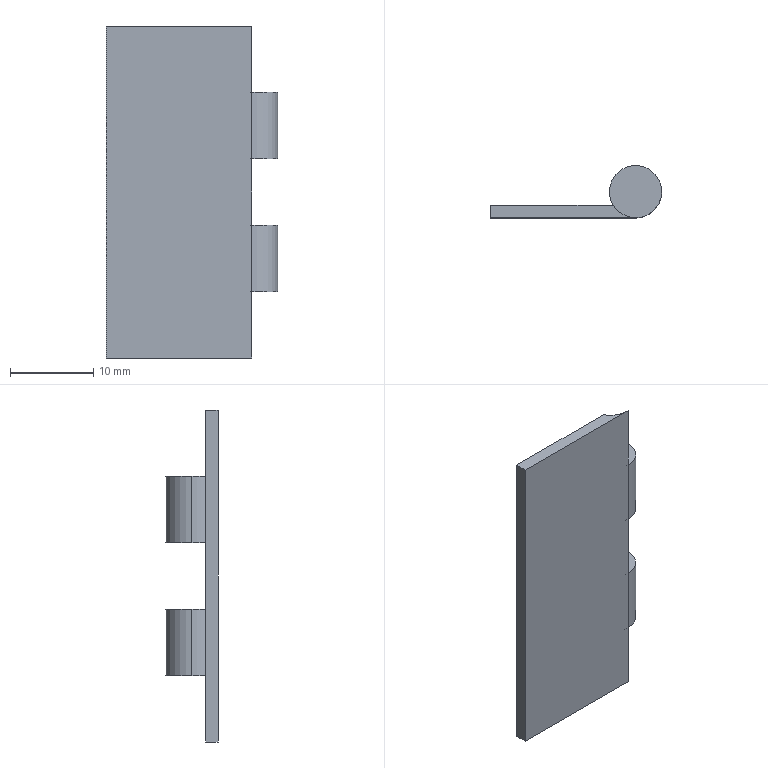Part | SolidWorks | features BaseBody 1 | 1 solid | 18 faces | box 20.65 x 6.3 x 40 mm | volume 1435 mm3 | cylinder 9 | plane 9 | commonest cylinder face diameters 6.3 x9
STEP:
#1=CARTESIAN_POINT('',(3.15,3.15,8.));
#2=VERTEX_POINT('',#1);
#3=CARTESIAN_POINT('',(-3.15,3.15,8.));
#4=VERTEX_POINT('',#3);
#5=CARTESIAN_POINT('',(0.,3.15,8.));
#6=DIRECTION('',(0.,0.,1.));
#7=DIRECTION('',(1.,0.,0.));
#8=AXIS2_PLACEMENT_3D('',#5,#6,#7);
#9=CIRCLE('',#8,3.15);
#10=EDGE_CURVE('',#2,#4,#9,.T.);
#11=ORIENTED_EDGE('',*,*,#10,.T.);
#12=CARTESIAN_POINT('',(-3.15,3.15,16.));
#13=VERTEX_POINT('',#12);
#14=CARTESIAN_POINT('',(-3.15,3.15,40.));
#15=DIRECTION('',(0.,0.,1.));
#16=VECTOR('',#15,1000.);
#17=LINE('',#14,#16);
#18=EDGE_CURVE('',#4,#13,#17,.T.);
#19=ORIENTED_EDGE('',*,*,#18,.T.);
#20=CARTESIAN_POINT('',(3.15,3.15,16.));
#21=VERTEX_POINT('',#20);
#22=CARTESIAN_POINT('',(0.,3.15,16.));
#23=DIRECTION('',(0.,0.,-1.));
#24=DIRECTION('',(1.,0.,0.));
#25=AXIS2_PLACEMENT_3D('',#22,#23,#24);
#26=CIRCLE('',#25,3.15);
#27=EDGE_CURVE('',#13,#21,#26,.T.);
#28=ORIENTED_EDGE('',*,*,#27,.T.);
#29=CARTESIAN_POINT('',(3.15,3.15,40.));
#30=DIRECTION('',(0.,0.,1.));
#31=VECTOR('',#30,1000.);
#32=LINE('',#29,#31);
#33=EDGE_CURVE('',#2,#21,#32,.T.);
#34=ORIENTED_EDGE('',*,*,#33,.F.);
#35=EDGE_LOOP('',(#11,#19,#28,#34));
#36=FACE_OUTER_BOUND('',#35,.T.);
#37=CARTESIAN_POINT('',(0.,3.15,40.));
#38=DIRECTION('',(0.,0.,1.));
#39=DIRECTION('',(1.,0.,0.));
#40=AXIS2_PLACEMENT_3D('',#37,#38,#39);
#41=CYLINDRICAL_SURFACE('',#40,3.15);
#42=ADVANCED_FACE('',(#36),#41,.T.);
#43=CARTESIAN_POINT('',(0.,0.,8.));
#44=VERTEX_POINT('',#43);
#45=CARTESIAN_POINT('',(0.,3.15,8.));
#46=DIRECTION('',(0.,0.,1.));
#47=DIRECTION('',(1.,0.,0.));
#48=AXIS2_PLACEMENT_3D('',#45,#46,#47);
#49=CIRCLE('',#48,3.15);
#50=EDGE_CURVE('',#44,#2,#49,.T.);
#51=ORIENTED_EDGE('',*,*,#50,.T.);
#52=ORIENTED_EDGE('',*,*,#33,.T.);
#53=CARTESIAN_POINT('',(0.,0.,16.));
#54=VERTEX_POINT('',#53);
#55=CARTESIAN_POINT('',(0.,3.15,16.));
#56=DIRECTION('',(0.,0.,-1.));
#57=DIRECTION('',(1.,0.,0.));
#58=AXIS2_PLACEMENT_3D('',#55,#56,#57);
#59=CIRCLE('',#58,3.15);
#60=EDGE_CURVE('',#21,#54,#59,.T.);
#61=ORIENTED_EDGE('',*,*,#60,.T.);
#62=CARTESIAN_POINT('',(0.,0.,40.));
#63=DIRECTION('',(0.,0.,-1.));
#64=VECTOR('',#63,1000.);
#65=LINE('',#62,#64);
#66=EDGE_CURVE('',#54,#44,#65,.T.);
#67=ORIENTED_EDGE('',*,*,#66,.T.);
#68=EDGE_LOOP('',(#51,#52,#61,#67));
#69=FACE_OUTER_BOUND('',#68,.T.);
#70=CARTESIAN_POINT('',(0.,3.15,40.));
#71=DIRECTION('',(0.,0.,1.));
#72=DIRECTION('',(1.,0.,0.));
#73=AXIS2_PLACEMENT_3D('',#70,#71,#72);
#74=CYLINDRICAL_SURFACE('',#73,3.15);
#75=ADVANCED_FACE('',(#69),#74,.T.);
#76=CARTESIAN_POINT('',(3.15,3.15,24.));
#77=VERTEX_POINT('',#76);
#78=CARTESIAN_POINT('',(-3.15,3.15,24.));
#79=VERTEX_POINT('',#78);
#80=CARTESIAN_POINT('',(0.,3.15,24.));
#81=DIRECTION('',(0.,0.,1.));
#82=DIRECTION('',(1.,0.,0.));
#83=AXIS2_PLACEMENT_3D('',#80,#81,#82);
#84=CIRCLE('',#83,3.15);
#85=EDGE_CURVE('',#77,#79,#84,.T.);
#86=ORIENTED_EDGE('',*,*,#85,.T.);
#87=CARTESIAN_POINT('',(-3.15,3.15,32.));
#88=VERTEX_POINT('',#87);
#89=CARTESIAN_POINT('',(-3.15,3.15,40.));
#90=DIRECTION('',(0.,0.,1.));
#91=VECTOR('',#90,1000.);
#92=LINE('',#89,#91);
#93=EDGE_CURVE('',#79,#88,#92,.T.);
#94=ORIENTED_EDGE('',*,*,#93,.T.);
#95=CARTESIAN_POINT('',(3.15,3.15,32.));
#96=VERTEX_POINT('',#95);
#97=CARTESIAN_POINT('',(0.,3.15,32.));
#98=DIRECTION('',(0.,0.,-1.));
#99=DIRECTION('',(1.,0.,0.));
#100=AXIS2_PLACEMENT_3D('',#97,#98,#99);
#101=CIRCLE('',#100,3.15);
#102=EDGE_CURVE('',#88,#96,#101,.T.);
#103=ORIENTED_EDGE('',*,*,#102,.T.);
#104=CARTESIAN_POINT('',(3.15,3.15,40.));
#105=DIRECTION('',(0.,0.,1.));
#106=VECTOR('',#105,1000.);
#107=LINE('',#104,#106);
#108=EDGE_CURVE('',#77,#96,#107,.T.);
#109=ORIENTED_EDGE('',*,*,#108,.F.);
#110=EDGE_LOOP('',(#86,#94,#103,#109));
#111=FACE_OUTER_BOUND('',#110,.T.);
#112=CARTESIAN_POINT('',(0.,3.15,40.));
#113=DIRECTION('',(0.,0.,1.));
#114=DIRECTION('',(1.,0.,0.));
#115=AXIS2_PLACEMENT_3D('',#112,#113,#114);
#116=CYLINDRICAL_SURFACE('',#115,3.15);
#117=ADVANCED_FACE('',(#111),#116,.T.);
#118=CARTESIAN_POINT('',(0.,0.,24.));
#119=VERTEX_POINT('',#118);
#120=CARTESIAN_POINT('',(0.,3.15,24.));
#121=DIRECTION('',(0.,0.,1.));
#122=DIRECTION('',(1.,0.,0.));
#123=AXIS2_PLACEMENT_3D('',#120,#121,#122);
#124=CIRCLE('',#123,3.15);
#125=EDGE_CURVE('',#119,#77,#124,.T.);
#126=ORIENTED_EDGE('',*,*,#125,.T.);
#127=ORIENTED_EDGE('',*,*,#108,.T.);
#128=CARTESIAN_POINT('',(0.,0.,32.));
#129=VERTEX_POINT('',#128);
#130=CARTESIAN_POINT('',(0.,3.15,32.));
#131=DIRECTION('',(0.,0.,-1.));
#132=DIRECTION('',(1.,0.,0.));
#133=AXIS2_PLACEMENT_3D('',#130,#131,#132);
#134=CIRCLE('',#133,3.15);
#135=EDGE_CURVE('',#96,#129,#134,.T.);
#136=ORIENTED_EDGE('',*,*,#135,.T.);
#137=CARTESIAN_POINT('',(0.,0.,40.));
#138=DIRECTION('',(0.,0.,-1.));
#139=VECTOR('',#138,1000.);
#140=LINE('',#137,#139);
#141=EDGE_CURVE('',#129,#119,#140,.T.);
#142=ORIENTED_EDGE('',*,*,#141,.T.);
#143=EDGE_LOOP('',(#126,#127,#136,#142));
#144=FACE_OUTER_BOUND('',#143,.T.);
#145=CARTESIAN_POINT('',(0.,3.15,40.));
#146=DIRECTION('',(0.,0.,1.));
#147=DIRECTION('',(1.,0.,0.));
#148=AXIS2_PLACEMENT_3D('',#145,#146,#147);
#149=CYLINDRICAL_SURFACE('',#148,3.15);
#150=ADVANCED_FACE('',(#144),#149,.T.);
#151=CARTESIAN_POINT('',(0.,0.,0.));
#152=VERTEX_POINT('',#151);
#153=CARTESIAN_POINT('',(0.,0.,40.));
#154=DIRECTION('',(0.,0.,-1.));
#155=VECTOR('',#154,1000.);
#156=LINE('',#153,#155);
#157=EDGE_CURVE('',#44,#152,#156,.T.);
#158=ORIENTED_EDGE('',*,*,#157,.F.);
#159=ORIENTED_EDGE('',*,*,#66,.F.);
#160=CARTESIAN_POINT('',(0.,0.,40.));
#161=DIRECTION('',(0.,0.,-1.));
#162=VECTOR('',#161,1000.);
#163=LINE('',#160,#162);
#164=EDGE_CURVE('',#119,#54,#163,.T.);
#165=ORIENTED_EDGE('',*,*,#164,.F.);
#166=ORIENTED_EDGE('',*,*,#141,.F.);
#167=CARTESIAN_POINT('',(0.,0.,40.));
#168=VERTEX_POINT('',#167);
#169=CARTESIAN_POINT('',(0.,0.,40.));
#170=DIRECTION('',(0.,0.,-1.));
#171=VECTOR('',#170,1000.);
#172=LINE('',#169,#171);
#173=EDGE_CURVE('',#168,#129,#172,.T.);
#174=ORIENTED_EDGE('',*,*,#173,.F.);
#175=CARTESIAN_POINT('',(-17.5,0.,40.));
#176=VERTEX_POINT('',#175);
#177=CARTESIAN_POINT('',(-17.5,0.,40.));
#178=DIRECTION('',(1.,0.,0.));
#179=VECTOR('',#178,1000.);
#180=LINE('',#177,#179);
#181=EDGE_CURVE('',#176,#168,#180,.T.);
#182=ORIENTED_EDGE('',*,*,#181,.F.);
#183=CARTESIAN_POINT('',(-17.5,0.,0.));
#184=VERTEX_POINT('',#183);
#185=CARTESIAN_POINT('',(-17.5,0.,40.));
#186=DIRECTION('',(0.,0.,1.));
#187=VECTOR('',#186,1000.);
#188=LINE('',#185,#187);
#189=EDGE_CURVE('',#184,#176,#188,.T.);
#190=ORIENTED_EDGE('',*,*,#189,.F.);
#191=CARTESIAN_POINT('',(-17.5,0.,0.));
#192=DIRECTION('',(-1.,0.,0.));
#193=VECTOR('',#192,1000.);
#194=LINE('',#191,#193);
#195=EDGE_CURVE('',#152,#184,#194,.T.);
#196=ORIENTED_EDGE('',*,*,#195,.F.);
#197=EDGE_LOOP('',(#158,#159,#165,#166,#174,#182,#190,#196));
#198=FACE_OUTER_BOUND('',#197,.T.);
#199=CARTESIAN_POINT('',(-17.5,0.,40.));
#200=DIRECTION('',(0.,1.,0.));
#201=DIRECTION('',(0.,0.,1.));
#202=AXIS2_PLACEMENT_3D('',#199,#200,#201);
#203=PLANE('',#202);
#204=ADVANCED_FACE('',(#198),#203,.F.);
#205=ORIENTED_EDGE('',*,*,#195,.T.);
#206=CARTESIAN_POINT('',(-17.5,1.5,0.));
#207=VERTEX_POINT('',#206);
#208=CARTESIAN_POINT('',(-17.5,3.15,0.));
#209=DIRECTION('',(0.,-1.,0.));
#210=VECTOR('',#209,1000.);
#211=LINE('',#208,#210);
#212=EDGE_CURVE('',#207,#184,#211,.T.);
#213=ORIENTED_EDGE('',*,*,#212,.F.);
#214=CARTESIAN_POINT('',(-2.683,1.5,0.));
#215=VERTEX_POINT('',#214);
#216=CARTESIAN_POINT('',(0.,1.5,0.));
#217=DIRECTION('',(-1.,0.,0.));
#218=VECTOR('',#217,1000.);
#219=LINE('',#216,#218);
#220=EDGE_CURVE('',#215,#207,#219,.T.);
#221=ORIENTED_EDGE('',*,*,#220,.F.);
#222=CARTESIAN_POINT('',(0.,3.15,0.));
#223=DIRECTION('',(0.,0.,-1.));
#224=DIRECTION('',(1.,0.,0.));
#225=AXIS2_PLACEMENT_3D('',#222,#223,#224);
#226=CIRCLE('',#225,3.15);
#227=EDGE_CURVE('',#152,#215,#226,.T.);
#228=ORIENTED_EDGE('',*,*,#227,.F.);
#229=EDGE_LOOP('',(#205,#213,#221,#228));
#230=FACE_OUTER_BOUND('',#229,.T.);
#231=CARTESIAN_POINT('',(0.,3.15,0.));
#232=DIRECTION('',(0.,0.,1.));
#233=DIRECTION('',(1.,0.,0.));
#234=AXIS2_PLACEMENT_3D('',#231,#232,#233);
#235=PLANE('',#234);
#236=ADVANCED_FACE('',(#230),#235,.F.);
#237=CARTESIAN_POINT('',(-2.683,1.5,8.));
#238=VERTEX_POINT('',#237);
#239=CARTESIAN_POINT('',(0.,3.15,8.));
#240=DIRECTION('',(0.,0.,-1.));
#241=DIRECTION('',(1.,0.,0.));
#242=AXIS2_PLACEMENT_3D('',#239,#240,#241);
#243=CIRCLE('',#242,3.15);
#244=EDGE_CURVE('',#44,#238,#243,.T.);
#245=ORIENTED_EDGE('',*,*,#244,.F.);
#246=ORIENTED_EDGE('',*,*,#157,.T.);
#247=ORIENTED_EDGE('',*,*,#227,.T.);
#248=CARTESIAN_POINT('',(-2.683,1.5,8.));
#249=DIRECTION('',(0.,0.,-1.));
#250=VECTOR('',#249,1000.);
#251=LINE('',#248,#250);
#252=EDGE_CURVE('',#238,#215,#251,.T.);
#253=ORIENTED_EDGE('',*,*,#252,.F.);
#254=EDGE_LOOP('',(#245,#246,#247,#253));
#255=FACE_OUTER_BOUND('',#254,.T.);
#256=CARTESIAN_POINT('',(0.,3.15,8.));
#257=DIRECTION('',(0.,0.,1.));
#258=DIRECTION('',(1.,0.,0.));
#259=AXIS2_PLACEMENT_3D('',#256,#257,#258);
#260=CYLINDRICAL_SURFACE('',#259,3.15);
#261=ADVANCED_FACE('',(#255),#260,.F.);
#262=ORIENTED_EDGE('',*,*,#18,.F.);
#263=CARTESIAN_POINT('',(0.,3.15,8.));
#264=DIRECTION('',(0.,0.,1.));
#265=DIRECTION('',(1.,0.,0.));
#266=AXIS2_PLACEMENT_3D('',#263,#264,#265);
#267=CIRCLE('',#266,3.15);
#268=EDGE_CURVE('',#4,#238,#267,.T.);
#269=ORIENTED_EDGE('',*,*,#268,.T.);
#270=CARTESIAN_POINT('',(-2.683,1.5,16.));
#271=VERTEX_POINT('',#270);
#272=CARTESIAN_POINT('',(-2.683,1.5,40.));
#273=DIRECTION('',(0.,0.,1.));
#274=VECTOR('',#273,1000.);
#275=LINE('',#272,#274);
#276=EDGE_CURVE('',#238,#271,#275,.T.);
#277=ORIENTED_EDGE('',*,*,#276,.T.);
#278=CARTESIAN_POINT('',(0.,3.15,16.));
#279=DIRECTION('',(0.,0.,-1.));
#280=DIRECTION('',(1.,0.,0.));
#281=AXIS2_PLACEMENT_3D('',#278,#279,#280);
#282=CIRCLE('',#281,3.15);
#283=EDGE_CURVE('',#271,#13,#282,.T.);
#284=ORIENTED_EDGE('',*,*,#283,.T.);
#285=EDGE_LOOP('',(#262,#269,#277,#284));
#286=FACE_OUTER_BOUND('',#285,.T.);
#287=CARTESIAN_POINT('',(0.,3.15,40.));
#288=DIRECTION('',(0.,0.,1.));
#289=DIRECTION('',(1.,0.,0.));
#290=AXIS2_PLACEMENT_3D('',#287,#288,#289);
#291=CYLINDRICAL_SURFACE('',#290,3.15);
#292=ADVANCED_FACE('',(#286),#291,.T.);
#293=CARTESIAN_POINT('',(-2.683,1.5,24.));
#294=VERTEX_POINT('',#293);
#295=CARTESIAN_POINT('',(0.,3.15,24.));
#296=DIRECTION('',(0.,0.,-1.));
#297=DIRECTION('',(1.,0.,0.));
#298=AXIS2_PLACEMENT_3D('',#295,#296,#297);
#299=CIRCLE('',#298,3.15);
#300=EDGE_CURVE('',#119,#294,#299,.T.);
#301=ORIENTED_EDGE('',*,*,#300,.F.);
#302=ORIENTED_EDGE('',*,*,#164,.T.);
#303=CARTESIAN_POINT('',(0.,3.15,16.));
#304=DIRECTION('',(0.,0.,1.));
#305=DIRECTION('',(1.,0.,0.));
#306=AXIS2_PLACEMENT_3D('',#303,#304,#305);
#307=CIRCLE('',#306,3.15);
#308=EDGE_CURVE('',#271,#54,#307,.T.);
#309=ORIENTED_EDGE('',*,*,#308,.F.);
#310=CARTESIAN_POINT('',(-2.683,1.5,24.));
#311=DIRECTION('',(0.,0.,-1.));
#312=VECTOR('',#311,1000.);
#313=LINE('',#310,#312);
#314=EDGE_CURVE('',#294,#271,#313,.T.);
#315=ORIENTED_EDGE('',*,*,#314,.F.);
#316=EDGE_LOOP('',(#301,#302,#309,#315));
#317=FACE_OUTER_BOUND('',#316,.T.);
#318=CARTESIAN_POINT('',(0.,3.15,24.));
#319=DIRECTION('',(0.,0.,1.));
#320=DIRECTION('',(1.,0.,0.));
#321=AXIS2_PLACEMENT_3D('',#318,#319,#320);
#322=CYLINDRICAL_SURFACE('',#321,3.15);
#323=ADVANCED_FACE('',(#317),#322,.F.);
#324=ORIENTED_EDGE('',*,*,#93,.F.);
#325=CARTESIAN_POINT('',(0.,3.15,24.));
#326=DIRECTION('',(0.,0.,1.));
#327=DIRECTION('',(1.,0.,0.));
#328=AXIS2_PLACEMENT_3D('',#325,#326,#327);
#329=CIRCLE('',#328,3.15);
#330=EDGE_CURVE('',#79,#294,#329,.T.);
#331=ORIENTED_EDGE('',*,*,#330,.T.);
#332=CARTESIAN_POINT('',(-2.683,1.5,32.));
#333=VERTEX_POINT('',#332);
#334=CARTESIAN_POINT('',(-2.683,1.5,40.));
#335=DIRECTION('',(0.,0.,1.));
#336=VECTOR('',#335,1000.);
#337=LINE('',#334,#336);
#338=EDGE_CURVE('',#294,#333,#337,.T.);
#339=ORIENTED_EDGE('',*,*,#338,.T.);
#340=CARTESIAN_POINT('',(0.,3.15,32.));
#341=DIRECTION('',(0.,0.,-1.));
#342=DIRECTION('',(1.,0.,0.));
#343=AXIS2_PLACEMENT_3D('',#340,#341,#342);
#344=CIRCLE('',#343,3.15);
#345=EDGE_CURVE('',#333,#88,#344,.T.);
#346=ORIENTED_EDGE('',*,*,#345,.T.);
#347=EDGE_LOOP('',(#324,#331,#339,#346));
#348=FACE_OUTER_BOUND('',#347,.T.);
#349=CARTESIAN_POINT('',(0.,3.15,40.));
#350=DIRECTION('',(0.,0.,1.));
#351=DIRECTION('',(1.,0.,0.));
#352=AXIS2_PLACEMENT_3D('',#349,#350,#351);
#353=CYLINDRICAL_SURFACE('',#352,3.15);
#354=ADVANCED_FACE('',(#348),#353,.T.);
#355=CARTESIAN_POINT('',(-2.683,1.5,40.));
#356=VERTEX_POINT('',#355);
#357=CARTESIAN_POINT('',(0.,3.15,40.));
#358=DIRECTION('',(0.,0.,-1.));
#359=DIRECTION('',(1.,0.,0.));
#360=AXIS2_PLACEMENT_3D('',#357,#358,#359);
#361=CIRCLE('',#360,3.15);
#362=EDGE_CURVE('',#168,#356,#361,.T.);
#363=ORIENTED_EDGE('',*,*,#362,.F.);
#364=ORIENTED_EDGE('',*,*,#173,.T.);
#365=CARTESIAN_POINT('',(0.,3.15,32.));
#366=DIRECTION('',(0.,0.,1.));
#367=DIRECTION('',(1.,0.,0.));
#368=AXIS2_PLACEMENT_3D('',#365,#366,#367);
#369=CIRCLE('',#368,3.15);
#370=EDGE_CURVE('',#333,#129,#369,.T.);
#371=ORIENTED_EDGE('',*,*,#370,.F.);
#372=CARTESIAN_POINT('',(-2.683,1.5,40.));
#373=DIRECTION('',(0.,0.,-1.));
#374=VECTOR('',#373,1000.);
#375=LINE('',#372,#374);
#376=EDGE_CURVE('',#356,#333,#375,.T.);
#377=ORIENTED_EDGE('',*,*,#376,.F.);
#378=EDGE_LOOP('',(#363,#364,#371,#377));
#379=FACE_OUTER_BOUND('',#378,.T.);
#380=CARTESIAN_POINT('',(0.,3.15,40.));
#381=DIRECTION('',(0.,0.,1.));
#382=DIRECTION('',(1.,0.,0.));
#383=AXIS2_PLACEMENT_3D('',#380,#381,#382);
#384=CYLINDRICAL_SURFACE('',#383,3.15);
#385=ADVANCED_FACE('',(#379),#384,.F.);
#386=CARTESIAN_POINT('',(-17.5,1.5,40.));
#387=VERTEX_POINT('',#386);
#388=CARTESIAN_POINT('',(0.,1.5,40.));
#389=DIRECTION('',(-1.,0.,0.));
#390=VECTOR('',#389,1000.);
#391=LINE('',#388,#390);
#392=EDGE_CURVE('',#356,#387,#391,.T.);
#393=ORIENTED_EDGE('',*,*,#392,.T.);
#394=CARTESIAN_POINT('',(-17.5,3.15,40.));
#395=DIRECTION('',(0.,-1.,0.));
#396=VECTOR('',#395,1000.);
#397=LINE('',#394,#396);
#398=EDGE_CURVE('',#387,#176,#397,.T.);
#399=ORIENTED_EDGE('',*,*,#398,.T.);
#400=ORIENTED_EDGE('',*,*,#181,.T.);
#401=ORIENTED_EDGE('',*,*,#362,.T.);
#402=EDGE_LOOP('',(#393,#399,#400,#401));
#403=FACE_OUTER_BOUND('',#402,.T.);
#404=CARTESIAN_POINT('',(0.,3.15,40.));
#405=DIRECTION('',(0.,0.,1.));
#406=DIRECTION('',(1.,0.,0.));
#407=AXIS2_PLACEMENT_3D('',#404,#405,#406);
#408=PLANE('',#407);
#409=ADVANCED_FACE('',(#403),#408,.T.);
#410=ORIENTED_EDGE('',*,*,#189,.T.);
#411=ORIENTED_EDGE('',*,*,#398,.F.);
#412=CARTESIAN_POINT('',(-17.5,1.5,40.));
#413=DIRECTION('',(0.,0.,1.));
#414=VECTOR('',#413,1000.);
#415=LINE('',#412,#414);
#416=EDGE_CURVE('',#207,#387,#415,.T.);
#417=ORIENTED_EDGE('',*,*,#416,.F.);
#418=ORIENTED_EDGE('',*,*,#212,.T.);
#419=EDGE_LOOP('',(#410,#411,#417,#418));
#420=FACE_OUTER_BOUND('',#419,.T.);
#421=CARTESIAN_POINT('',(-17.5,1.5,40.));
#422=DIRECTION('',(1.,0.,0.));
#423=DIRECTION('',(0.,0.,-1.));
#424=AXIS2_PLACEMENT_3D('',#421,#422,#423);
#425=PLANE('',#424);
#426=ADVANCED_FACE('',(#420),#425,.F.);
#427=ORIENTED_EDGE('',*,*,#416,.T.);
#428=ORIENTED_EDGE('',*,*,#392,.F.);
#429=ORIENTED_EDGE('',*,*,#376,.T.);
#430=ORIENTED_EDGE('',*,*,#338,.F.);
#431=ORIENTED_EDGE('',*,*,#314,.T.);
#432=ORIENTED_EDGE('',*,*,#276,.F.);
#433=ORIENTED_EDGE('',*,*,#252,.T.);
#434=ORIENTED_EDGE('',*,*,#220,.T.);
#435=EDGE_LOOP('',(#427,#428,#429,#430,#431,#432,#433,#434));
#436=FACE_OUTER_BOUND('',#435,.T.);
#437=CARTESIAN_POINT('',(-2.683,1.5,40.));
#438=DIRECTION('',(0.,-1.,0.));
#439=DIRECTION('',(0.,0.,-1.));
#440=AXIS2_PLACEMENT_3D('',#437,#438,#439);
#441=PLANE('',#440);
#442=ADVANCED_FACE('',(#436),#441,.F.);
#443=ORIENTED_EDGE('',*,*,#50,.F.);
#444=ORIENTED_EDGE('',*,*,#244,.T.);
#445=ORIENTED_EDGE('',*,*,#268,.F.);
#446=ORIENTED_EDGE('',*,*,#10,.F.);
#447=EDGE_LOOP('',(#443,#444,#445,#446));
#448=FACE_OUTER_BOUND('',#447,.T.);
#449=CARTESIAN_POINT('',(0.,3.15,8.));
#450=DIRECTION('',(0.,0.,1.));
#451=DIRECTION('',(1.,0.,0.));
#452=AXIS2_PLACEMENT_3D('',#449,#450,#451);
#453=PLANE('',#452);
#454=ADVANCED_FACE('',(#448),#453,.F.);
#455=ORIENTED_EDGE('',*,*,#308,.T.);
#456=ORIENTED_EDGE('',*,*,#60,.F.);
#457=ORIENTED_EDGE('',*,*,#27,.F.);
#458=ORIENTED_EDGE('',*,*,#283,.F.);
#459=EDGE_LOOP('',(#455,#456,#457,#458));
#460=FACE_OUTER_BOUND('',#459,.T.);
#461=CARTESIAN_POINT('',(0.,3.15,16.));
#462=DIRECTION('',(0.,0.,1.));
#463=DIRECTION('',(1.,0.,0.));
#464=AXIS2_PLACEMENT_3D('',#461,#462,#463);
#465=PLANE('',#464);
#466=ADVANCED_FACE('',(#460),#465,.T.);
#467=ORIENTED_EDGE('',*,*,#125,.F.);
#468=ORIENTED_EDGE('',*,*,#300,.T.);
#469=ORIENTED_EDGE('',*,*,#330,.F.);
#470=ORIENTED_EDGE('',*,*,#85,.F.);
#471=EDGE_LOOP('',(#467,#468,#469,#470));
#472=FACE_OUTER_BOUND('',#471,.T.);
#473=CARTESIAN_POINT('',(0.,3.15,24.));
#474=DIRECTION('',(0.,0.,1.));
#475=DIRECTION('',(1.,0.,0.));
#476=AXIS2_PLACEMENT_3D('',#473,#474,#475);
#477=PLANE('',#476);
#478=ADVANCED_FACE('',(#472),#477,.F.);
#479=ORIENTED_EDGE('',*,*,#370,.T.);
#480=ORIENTED_EDGE('',*,*,#135,.F.);
#481=ORIENTED_EDGE('',*,*,#102,.F.);
#482=ORIENTED_EDGE('',*,*,#345,.F.);
#483=EDGE_LOOP('',(#479,#480,#481,#482));
#484=FACE_OUTER_BOUND('',#483,.T.);
#485=CARTESIAN_POINT('',(0.,3.15,32.));
#486=DIRECTION('',(0.,0.,1.));
#487=DIRECTION('',(1.,0.,0.));
#488=AXIS2_PLACEMENT_3D('',#485,#486,#487);
#489=PLANE('',#488);
#490=ADVANCED_FACE('',(#484),#489,.T.);
#491=CLOSED_SHELL('',(#42,#75,#117,#150,#204,#236,#261,#292,#323,#354,#385,#409,#426,#442,#454,#466,#478,#490));
#492=MANIFOLD_SOLID_BREP('',#491);
#493=CARTESIAN_POINT('',(0.,0.,0.));
#494=DIRECTION('',(0.,0.,1.));
#495=DIRECTION('',(1.,0.,0.));
#496=AXIS2_PLACEMENT_3D('',#493,#494,#495);
#497=(LENGTH_UNIT()NAMED_UNIT(*)SI_UNIT(.MILLI.,.METRE.));
#498=UNCERTAINTY_MEASURE_WITH_UNIT(LENGTH_MEASURE(0.00001),#497,'','');
#499=(NAMED_UNIT(*)PLANE_ANGLE_UNIT()SI_UNIT($,.RADIAN.));
#500=(NAMED_UNIT(*)SI_UNIT($,.STERADIAN.)SOLID_ANGLE_UNIT());
#501=(GEOMETRIC_REPRESENTATION_CONTEXT(3)GLOBAL_UNCERTAINTY_ASSIGNED_CONTEXT((#498))GLOBAL_UNIT_ASSIGNED_CONTEXT((#497,#499,#500))REPRESENTATION_CONTEXT('',''));
#502=ADVANCED_BREP_SHAPE_REPRESENTATION('',(#492,#496),#501);